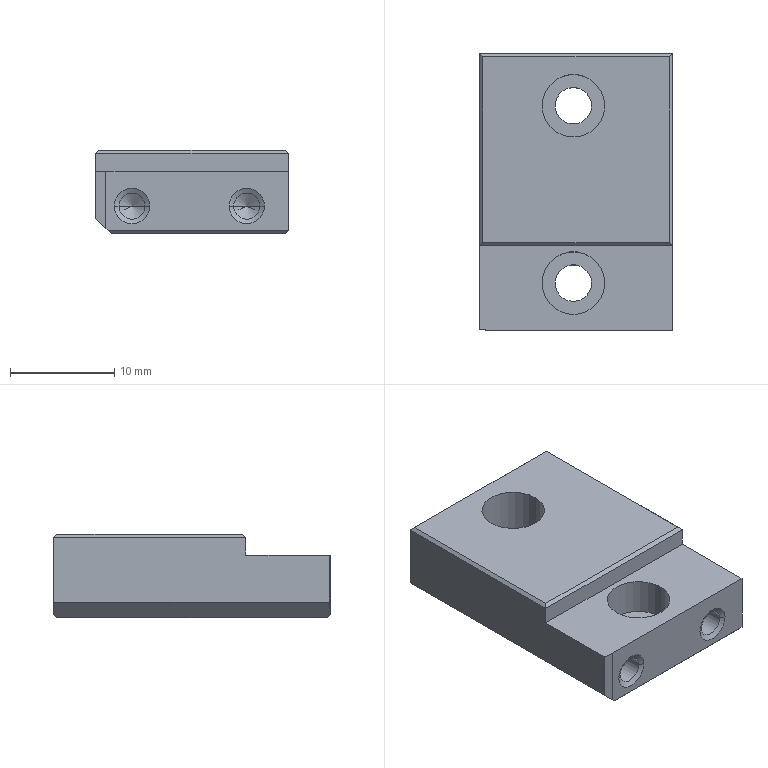Part | NX | 1 solid | 39 faces | box 18.5 x 26.53 x 8 mm | volume 3216 mm3 | plane 19 | cylinder 12 | cone 8 | commonest cylinder face diameters 2.5 x4 3.5 x4 6 x4
STEP:
#1=CARTESIAN_POINT('',(0.3,26.23,8.));
#2=VERTEX_POINT('',#1);
#3=CARTESIAN_POINT('',(0.3,8.4,8.));
#4=VERTEX_POINT('',#3);
#5=CARTESIAN_POINT('',(0.3,0.,8.));
#6=DIRECTION('',(0.,-1.,0.));
#7=VECTOR('',#6,1000.);
#8=LINE('',#5,#7);
#9=EDGE_CURVE('',#2,#4,#8,.T.);
#10=ORIENTED_EDGE('',*,*,#9,.T.);
#11=CARTESIAN_POINT('',(18.2,8.4,8.));
#12=VERTEX_POINT('',#11);
#13=CARTESIAN_POINT('',(0.,8.4,8.));
#14=DIRECTION('',(-1.,0.,0.));
#15=VECTOR('',#14,1000.);
#16=LINE('',#13,#15);
#17=EDGE_CURVE('',#12,#4,#16,.T.);
#18=ORIENTED_EDGE('',*,*,#17,.F.);
#19=CARTESIAN_POINT('',(18.2,26.23,8.));
#20=VERTEX_POINT('',#19);
#21=CARTESIAN_POINT('',(18.2,0.,8.));
#22=DIRECTION('',(0.,-1.,0.));
#23=VECTOR('',#22,1000.);
#24=LINE('',#21,#23);
#25=EDGE_CURVE('',#20,#12,#24,.T.);
#26=ORIENTED_EDGE('',*,*,#25,.F.);
#27=CARTESIAN_POINT('',(0.,26.23,8.));
#28=DIRECTION('',(1.,0.,0.));
#29=VECTOR('',#28,1000.);
#30=LINE('',#27,#29);
#31=EDGE_CURVE('',#2,#20,#30,.T.);
#32=ORIENTED_EDGE('',*,*,#31,.F.);
#33=EDGE_LOOP('',(#10,#18,#26,#32));
#34=FACE_BOUND('',#33,.T.);
#35=CARTESIAN_POINT('',(12.,21.53,8.));
#36=VERTEX_POINT('',#35);
#37=CARTESIAN_POINT('',(6.,21.53,8.));
#38=VERTEX_POINT('',#37);
#39=CARTESIAN_POINT('',(9.,21.53,8.));
#40=DIRECTION('',(0.,0.,1.));
#41=DIRECTION('',(1.,0.,0.));
#42=AXIS2_PLACEMENT_3D('',#39,#40,#41);
#43=CIRCLE('',#42,3.);
#44=EDGE_CURVE('',#36,#38,#43,.T.);
#45=ORIENTED_EDGE('',*,*,#44,.F.);
#46=CARTESIAN_POINT('',(9.,21.53,8.));
#47=DIRECTION('',(0.,0.,1.));
#48=DIRECTION('',(1.,0.,0.));
#49=AXIS2_PLACEMENT_3D('',#46,#47,#48);
#50=CIRCLE('',#49,3.);
#51=EDGE_CURVE('',#38,#36,#50,.T.);
#52=ORIENTED_EDGE('',*,*,#51,.F.);
#53=EDGE_LOOP('',(#45,#52));
#54=FACE_BOUND('',#53,.T.);
#55=CARTESIAN_POINT('',(0.,0.,8.));
#56=DIRECTION('',(0.,0.,1.));
#57=DIRECTION('',(1.,0.,0.));
#58=AXIS2_PLACEMENT_3D('',#55,#56,#57);
#59=PLANE('',#58);
#60=ADVANCED_FACE('',(#34,#54),#59,.T.);
#61=CARTESIAN_POINT('',(12.,4.53,2.5));
#62=VERTEX_POINT('',#61);
#63=CARTESIAN_POINT('',(6.,4.53,2.5));
#64=VERTEX_POINT('',#63);
#65=CARTESIAN_POINT('',(9.,4.53,2.5));
#66=DIRECTION('',(0.,0.,1.));
#67=DIRECTION('',(-1.,0.,0.));
#68=AXIS2_PLACEMENT_3D('',#65,#66,#67);
#69=CIRCLE('',#68,3.);
#70=EDGE_CURVE('',#62,#64,#69,.T.);
#71=ORIENTED_EDGE('',*,*,#70,.T.);
#72=CARTESIAN_POINT('',(9.,4.53,2.5));
#73=DIRECTION('',(0.,0.,1.));
#74=DIRECTION('',(-1.,0.,0.));
#75=AXIS2_PLACEMENT_3D('',#72,#73,#74);
#76=CIRCLE('',#75,3.);
#77=EDGE_CURVE('',#64,#62,#76,.T.);
#78=ORIENTED_EDGE('',*,*,#77,.T.);
#79=EDGE_LOOP('',(#71,#78));
#80=FACE_BOUND('',#79,.T.);
#81=CARTESIAN_POINT('',(7.25,4.53,2.5));
#82=VERTEX_POINT('',#81);
#83=CARTESIAN_POINT('',(10.75,4.53,2.5));
#84=VERTEX_POINT('',#83);
#85=CARTESIAN_POINT('',(9.,4.53,2.5));
#86=DIRECTION('',(0.,0.,1.));
#87=DIRECTION('',(-1.,0.,0.));
#88=AXIS2_PLACEMENT_3D('',#85,#86,#87);
#89=CIRCLE('',#88,1.75);
#90=EDGE_CURVE('',#82,#84,#89,.T.);
#91=ORIENTED_EDGE('',*,*,#90,.F.);
#92=CARTESIAN_POINT('',(9.,4.53,2.5));
#93=DIRECTION('',(0.,0.,1.));
#94=DIRECTION('',(-1.,0.,0.));
#95=AXIS2_PLACEMENT_3D('',#92,#93,#94);
#96=CIRCLE('',#95,1.75);
#97=EDGE_CURVE('',#84,#82,#96,.T.);
#98=ORIENTED_EDGE('',*,*,#97,.F.);
#99=EDGE_LOOP('',(#91,#98));
#100=FACE_BOUND('',#99,.T.);
#101=CARTESIAN_POINT('',(9.,4.53,2.5));
#102=DIRECTION('',(0.,0.,1.));
#103=DIRECTION('',(1.,0.,0.));
#104=AXIS2_PLACEMENT_3D('',#101,#102,#103);
#105=PLANE('',#104);
#106=ADVANCED_FACE('',(#80,#100),#105,.T.);
#107=CARTESIAN_POINT('',(18.5,0.,6.));
#108=VERTEX_POINT('',#107);
#109=CARTESIAN_POINT('',(1.,0.,6.));
#110=VERTEX_POINT('',#109);
#111=CARTESIAN_POINT('',(0.,0.,6.));
#112=DIRECTION('',(-1.,0.,0.));
#113=VECTOR('',#112,1000.);
#114=LINE('',#111,#113);
#115=EDGE_CURVE('',#108,#110,#114,.T.);
#116=ORIENTED_EDGE('',*,*,#115,.T.);
#117=CARTESIAN_POINT('',(1.,0.,0.5));
#118=VERTEX_POINT('',#117);
#119=CARTESIAN_POINT('',(1.,0.,0.));
#120=DIRECTION('',(0.,0.,1.));
#121=VECTOR('',#120,1000.);
#122=LINE('',#119,#121);
#123=EDGE_CURVE('',#118,#110,#122,.T.);
#124=ORIENTED_EDGE('',*,*,#123,.F.);
#125=CARTESIAN_POINT('',(1.2,0.,0.3));
#126=VERTEX_POINT('',#125);
#127=CARTESIAN_POINT('',(1.5,0.,0.));
#128=DIRECTION('',(-0.7071,0.,0.7071));
#129=VECTOR('',#128,1000.);
#130=LINE('',#127,#129);
#131=EDGE_CURVE('',#126,#118,#130,.T.);
#132=ORIENTED_EDGE('',*,*,#131,.F.);
#133=CARTESIAN_POINT('',(18.5,0.,0.3));
#134=VERTEX_POINT('',#133);
#135=CARTESIAN_POINT('',(0.,0.,0.3));
#136=DIRECTION('',(1.,0.,0.));
#137=VECTOR('',#136,1000.);
#138=LINE('',#135,#137);
#139=EDGE_CURVE('',#126,#134,#138,.T.);
#140=ORIENTED_EDGE('',*,*,#139,.T.);
#141=CARTESIAN_POINT('',(18.5,0.,0.));
#142=DIRECTION('',(0.,0.,-1.));
#143=VECTOR('',#142,1000.);
#144=LINE('',#141,#143);
#145=EDGE_CURVE('',#108,#134,#144,.T.);
#146=ORIENTED_EDGE('',*,*,#145,.F.);
#147=EDGE_LOOP('',(#116,#124,#132,#140,#146));
#148=FACE_BOUND('',#147,.T.);
#149=CARTESIAN_POINT('',(12.8,0.,2.65));
#150=VERTEX_POINT('',#149);
#151=CARTESIAN_POINT('',(16.2,0.,2.65));
#152=VERTEX_POINT('',#151);
#153=CARTESIAN_POINT('',(14.5,0.,2.65));
#154=DIRECTION('',(0.,-1.,0.));
#155=DIRECTION('',(-1.,0.,0.));
#156=AXIS2_PLACEMENT_3D('',#153,#154,#155);
#157=CIRCLE('',#156,1.7);
#158=EDGE_CURVE('',#150,#152,#157,.T.);
#159=ORIENTED_EDGE('',*,*,#158,.F.);
#160=CARTESIAN_POINT('',(14.5,0.,2.65));
#161=DIRECTION('',(0.,-1.,0.));
#162=DIRECTION('',(-1.,0.,0.));
#163=AXIS2_PLACEMENT_3D('',#160,#161,#162);
#164=CIRCLE('',#163,1.7);
#165=EDGE_CURVE('',#152,#150,#164,.T.);
#166=ORIENTED_EDGE('',*,*,#165,.F.);
#167=EDGE_LOOP('',(#159,#166));
#168=FACE_BOUND('',#167,.T.);
#169=CARTESIAN_POINT('',(1.8,0.,2.65));
#170=VERTEX_POINT('',#169);
#171=CARTESIAN_POINT('',(5.2,0.,2.65));
#172=VERTEX_POINT('',#171);
#173=CARTESIAN_POINT('',(3.5,0.,2.65));
#174=DIRECTION('',(0.,-1.,0.));
#175=DIRECTION('',(-1.,0.,0.));
#176=AXIS2_PLACEMENT_3D('',#173,#174,#175);
#177=CIRCLE('',#176,1.7);
#178=EDGE_CURVE('',#170,#172,#177,.T.);
#179=ORIENTED_EDGE('',*,*,#178,.F.);
#180=CARTESIAN_POINT('',(3.5,0.,2.65));
#181=DIRECTION('',(0.,-1.,0.));
#182=DIRECTION('',(-1.,0.,0.));
#183=AXIS2_PLACEMENT_3D('',#180,#181,#182);
#184=CIRCLE('',#183,1.7);
#185=EDGE_CURVE('',#172,#170,#184,.T.);
#186=ORIENTED_EDGE('',*,*,#185,.F.);
#187=EDGE_LOOP('',(#179,#186));
#188=FACE_BOUND('',#187,.T.);
#189=CARTESIAN_POINT('',(0.,0.,0.));
#190=DIRECTION('',(0.,-1.,0.));
#191=DIRECTION('',(0.,0.,-1.));
#192=AXIS2_PLACEMENT_3D('',#189,#190,#191);
#193=PLANE('',#192);
#194=ADVANCED_FACE('',(#148,#168,#188),#193,.T.);
#195=ORIENTED_EDGE('',*,*,#123,.T.);
#196=CARTESIAN_POINT('',(0.,0.08749,6.));
#197=VERTEX_POINT('',#196);
#198=CARTESIAN_POINT('',(0.,0.08749,6.));
#199=DIRECTION('',(0.9962,-0.08716,0.));
#200=VECTOR('',#199,1000.);
#201=LINE('',#198,#200);
#202=EDGE_CURVE('',#197,#110,#201,.T.);
#203=ORIENTED_EDGE('',*,*,#202,.F.);
#204=CARTESIAN_POINT('',(0.,0.08749,1.5));
#205=VERTEX_POINT('',#204);
#206=CARTESIAN_POINT('',(0.,0.08749,0.));
#207=DIRECTION('',(0.,0.,-1.));
#208=VECTOR('',#207,1000.);
#209=LINE('',#206,#208);
#210=EDGE_CURVE('',#197,#205,#209,.T.);
#211=ORIENTED_EDGE('',*,*,#210,.T.);
#212=CARTESIAN_POINT('',(0.,0.08749,1.5));
#213=DIRECTION('',(-0.7058,0.06175,0.7058));
#214=VECTOR('',#213,1000.);
#215=LINE('',#212,#214);
#216=EDGE_CURVE('',#118,#205,#215,.T.);
#217=ORIENTED_EDGE('',*,*,#216,.F.);
#218=EDGE_LOOP('',(#195,#203,#211,#217));
#219=FACE_BOUND('',#218,.T.);
#220=CARTESIAN_POINT('',(1.,0.,0.5));
#221=DIRECTION('',(-0.08716,-0.9962,0.));
#222=DIRECTION('',(-0.9962,0.08716,0.));
#223=AXIS2_PLACEMENT_3D('',#220,#221,#222);
#224=PLANE('',#223);
#225=ADVANCED_FACE('',(#219),#224,.T.);
#226=CARTESIAN_POINT('',(1.5,0.3,0.));
#227=VERTEX_POINT('',#226);
#228=CARTESIAN_POINT('',(1.5,26.23,0.));
#229=VERTEX_POINT('',#228);
#230=CARTESIAN_POINT('',(1.5,0.,0.));
#231=DIRECTION('',(0.,1.,0.));
#232=VECTOR('',#231,1000.);
#233=LINE('',#230,#232);
#234=EDGE_CURVE('',#227,#229,#233,.T.);
#235=ORIENTED_EDGE('',*,*,#234,.F.);
#236=CARTESIAN_POINT('',(1.5,0.3,0.));
#237=DIRECTION('',(-0.5774,-0.5774,0.5774));
#238=VECTOR('',#237,1000.);
#239=LINE('',#236,#238);
#240=EDGE_CURVE('',#227,#126,#239,.T.);
#241=ORIENTED_EDGE('',*,*,#240,.T.);
#242=ORIENTED_EDGE('',*,*,#131,.T.);
#243=ORIENTED_EDGE('',*,*,#216,.T.);
#244=CARTESIAN_POINT('',(0.,26.53,1.5));
#245=VERTEX_POINT('',#244);
#246=CARTESIAN_POINT('',(0.,0.,1.5));
#247=DIRECTION('',(0.,1.,0.));
#248=VECTOR('',#247,1000.);
#249=LINE('',#246,#248);
#250=EDGE_CURVE('',#205,#245,#249,.T.);
#251=ORIENTED_EDGE('',*,*,#250,.T.);
#252=CARTESIAN_POINT('',(1.2,26.53,0.3));
#253=VERTEX_POINT('',#252);
#254=CARTESIAN_POINT('',(0.,26.53,1.5));
#255=DIRECTION('',(0.7071,0.,-0.7071));
#256=VECTOR('',#255,1000.);
#257=LINE('',#254,#256);
#258=EDGE_CURVE('',#245,#253,#257,.T.);
#259=ORIENTED_EDGE('',*,*,#258,.T.);
#260=CARTESIAN_POINT('',(27.73,0.,-26.23));
#261=DIRECTION('',(-0.5774,0.5774,0.5774));
#262=VECTOR('',#261,1000.);
#263=LINE('',#260,#262);
#264=EDGE_CURVE('',#229,#253,#263,.T.);
#265=ORIENTED_EDGE('',*,*,#264,.F.);
#266=EDGE_LOOP('',(#235,#241,#242,#243,#251,#259,#265));
#267=FACE_BOUND('',#266,.T.);
#268=CARTESIAN_POINT('',(1.5,26.53,0.));
#269=DIRECTION('',(-0.7071,0.,-0.7071));
#270=DIRECTION('',(-0.7071,0.,0.7071));
#271=AXIS2_PLACEMENT_3D('',#268,#269,#270);
#272=PLANE('',#271);
#273=ADVANCED_FACE('',(#267),#272,.T.);
#274=CARTESIAN_POINT('',(18.5,26.53,7.7));
#275=VERTEX_POINT('',#274);
#276=CARTESIAN_POINT('',(0.,26.53,7.7));
#277=VERTEX_POINT('',#276);
#278=CARTESIAN_POINT('',(0.,26.53,7.7));
#279=DIRECTION('',(-1.,0.,0.));
#280=VECTOR('',#279,1000.);
#281=LINE('',#278,#280);
#282=EDGE_CURVE('',#275,#277,#281,.T.);
#283=ORIENTED_EDGE('',*,*,#282,.F.);
#284=CARTESIAN_POINT('',(18.5,26.53,0.3));
#285=VERTEX_POINT('',#284);
#286=CARTESIAN_POINT('',(18.5,26.53,0.));
#287=DIRECTION('',(0.,0.,-1.));
#288=VECTOR('',#287,1000.);
#289=LINE('',#286,#288);
#290=EDGE_CURVE('',#275,#285,#289,.T.);
#291=ORIENTED_EDGE('',*,*,#290,.T.);
#292=CARTESIAN_POINT('',(0.,26.53,0.3));
#293=DIRECTION('',(1.,0.,0.));
#294=VECTOR('',#293,1000.);
#295=LINE('',#292,#294);
#296=EDGE_CURVE('',#253,#285,#295,.T.);
#297=ORIENTED_EDGE('',*,*,#296,.F.);
#298=ORIENTED_EDGE('',*,*,#258,.F.);
#299=CARTESIAN_POINT('',(0.,26.53,0.));
#300=DIRECTION('',(0.,0.,1.));
#301=VECTOR('',#300,1000.);
#302=LINE('',#299,#301);
#303=EDGE_CURVE('',#245,#277,#302,.T.);
#304=ORIENTED_EDGE('',*,*,#303,.T.);
#305=EDGE_LOOP('',(#283,#291,#297,#298,#304));
#306=FACE_BOUND('',#305,.T.);
#307=CARTESIAN_POINT('',(18.5,26.53,0.));
#308=DIRECTION('',(0.,1.,0.));
#309=DIRECTION('',(1.,0.,0.));
#310=AXIS2_PLACEMENT_3D('',#307,#308,#309);
#311=PLANE('',#310);
#312=ADVANCED_FACE('',(#306),#311,.T.);
#313=CARTESIAN_POINT('',(18.5,8.1,7.7));
#314=VERTEX_POINT('',#313);
#315=CARTESIAN_POINT('',(18.5,0.,7.7));
#316=DIRECTION('',(0.,1.,0.));
#317=VECTOR('',#316,1000.);
#318=LINE('',#315,#317);
#319=EDGE_CURVE('',#314,#275,#318,.T.);
#320=ORIENTED_EDGE('',*,*,#319,.F.);
#321=CARTESIAN_POINT('',(18.5,8.1,6.));
#322=VERTEX_POINT('',#321);
#323=CARTESIAN_POINT('',(18.5,8.1,0.));
#324=DIRECTION('',(0.,0.,-1.));
#325=VECTOR('',#324,1000.);
#326=LINE('',#323,#325);
#327=EDGE_CURVE('',#314,#322,#326,.T.);
#328=ORIENTED_EDGE('',*,*,#327,.T.);
#329=CARTESIAN_POINT('',(18.5,0.,6.));
#330=DIRECTION('',(0.,1.,0.));
#331=VECTOR('',#330,1000.);
#332=LINE('',#329,#331);
#333=EDGE_CURVE('',#108,#322,#332,.T.);
#334=ORIENTED_EDGE('',*,*,#333,.F.);
#335=ORIENTED_EDGE('',*,*,#145,.T.);
#336=CARTESIAN_POINT('',(18.5,0.,0.3));
#337=DIRECTION('',(0.,-1.,0.));
#338=VECTOR('',#337,1000.);
#339=LINE('',#336,#338);
#340=EDGE_CURVE('',#285,#134,#339,.T.);
#341=ORIENTED_EDGE('',*,*,#340,.F.);
#342=ORIENTED_EDGE('',*,*,#290,.F.);
#343=EDGE_LOOP('',(#320,#328,#334,#335,#341,#342));
#344=FACE_BOUND('',#343,.T.);
#345=CARTESIAN_POINT('',(18.5,0.,0.));
#346=DIRECTION('',(1.,0.,0.));
#347=DIRECTION('',(0.,1.,0.));
#348=AXIS2_PLACEMENT_3D('',#345,#346,#347);
#349=PLANE('',#348);
#350=ADVANCED_FACE('',(#344),#349,.T.);
#351=CARTESIAN_POINT('',(0.,8.1,7.7));
#352=VERTEX_POINT('',#351);
#353=CARTESIAN_POINT('',(0.,8.1,7.7));
#354=DIRECTION('',(-1.,0.,0.));
#355=VECTOR('',#354,1000.);
#356=LINE('',#353,#355);
#357=EDGE_CURVE('',#314,#352,#356,.T.);
#358=ORIENTED_EDGE('',*,*,#357,.T.);
#359=CARTESIAN_POINT('',(0.,8.1,6.));
#360=VERTEX_POINT('',#359);
#361=CARTESIAN_POINT('',(0.,8.1,0.));
#362=DIRECTION('',(0.,0.,1.));
#363=VECTOR('',#362,1000.);
#364=LINE('',#361,#363);
#365=EDGE_CURVE('',#360,#352,#364,.T.);
#366=ORIENTED_EDGE('',*,*,#365,.F.);
#367=CARTESIAN_POINT('',(0.,8.1,6.));
#368=DIRECTION('',(-1.,0.,0.));
#369=VECTOR('',#368,1000.);
#370=LINE('',#367,#369);
#371=EDGE_CURVE('',#322,#360,#370,.T.);
#372=ORIENTED_EDGE('',*,*,#371,.F.);
#373=ORIENTED_EDGE('',*,*,#327,.F.);
#374=EDGE_LOOP('',(#358,#366,#372,#373));
#375=FACE_BOUND('',#374,.T.);
#376=CARTESIAN_POINT('',(18.5,8.1,5.85));
#377=DIRECTION('',(0.,1.,0.));
#378=DIRECTION('',(1.,0.,0.));
#379=AXIS2_PLACEMENT_3D('',#376,#377,#378);
#380=PLANE('',#379);
#381=ADVANCED_FACE('',(#375),#380,.F.);
#382=CARTESIAN_POINT('',(18.2,26.23,0.));
#383=VERTEX_POINT('',#382);
#384=CARTESIAN_POINT('',(18.2,0.3,0.));
#385=VERTEX_POINT('',#384);
#386=CARTESIAN_POINT('',(18.2,0.,0.));
#387=DIRECTION('',(0.,-1.,0.));
#388=VECTOR('',#387,1000.);
#389=LINE('',#386,#388);
#390=EDGE_CURVE('',#383,#385,#389,.T.);
#391=ORIENTED_EDGE('',*,*,#390,.T.);
#392=CARTESIAN_POINT('',(0.,0.3,0.));
#393=DIRECTION('',(1.,0.,0.));
#394=VECTOR('',#393,1000.);
#395=LINE('',#392,#394);
#396=EDGE_CURVE('',#227,#385,#395,.T.);
#397=ORIENTED_EDGE('',*,*,#396,.F.);
#398=ORIENTED_EDGE('',*,*,#234,.T.);
#399=CARTESIAN_POINT('',(0.,26.23,0.));
#400=DIRECTION('',(1.,0.,0.));
#401=VECTOR('',#400,1000.);
#402=LINE('',#399,#401);
#403=EDGE_CURVE('',#229,#383,#402,.T.);
#404=ORIENTED_EDGE('',*,*,#403,.T.);
#405=EDGE_LOOP('',(#391,#397,#398,#404));
#406=FACE_BOUND('',#405,.T.);
#407=CARTESIAN_POINT('',(10.75,21.53,0.));
#408=VERTEX_POINT('',#407);
#409=CARTESIAN_POINT('',(7.25,21.53,0.));
#410=VERTEX_POINT('',#409);
#411=CARTESIAN_POINT('',(9.,21.53,0.));
#412=DIRECTION('',(0.,0.,-1.));
#413=DIRECTION('',(-1.,0.,0.));
#414=AXIS2_PLACEMENT_3D('',#411,#412,#413);
#415=CIRCLE('',#414,1.75);
#416=EDGE_CURVE('',#408,#410,#415,.T.);
#417=ORIENTED_EDGE('',*,*,#416,.F.);
#418=CARTESIAN_POINT('',(9.,21.53,0.));
#419=DIRECTION('',(0.,0.,-1.));
#420=DIRECTION('',(-1.,0.,0.));
#421=AXIS2_PLACEMENT_3D('',#418,#419,#420);
#422=CIRCLE('',#421,1.75);
#423=EDGE_CURVE('',#410,#408,#422,.T.);
#424=ORIENTED_EDGE('',*,*,#423,.F.);
#425=EDGE_LOOP('',(#417,#424));
#426=FACE_BOUND('',#425,.T.);
#427=CARTESIAN_POINT('',(7.25,4.53,0.));
#428=VERTEX_POINT('',#427);
#429=CARTESIAN_POINT('',(10.75,4.53,0.));
#430=VERTEX_POINT('',#429);
#431=CARTESIAN_POINT('',(9.,4.53,0.));
#432=DIRECTION('',(0.,0.,-1.));
#433=DIRECTION('',(-1.,0.,0.));
#434=AXIS2_PLACEMENT_3D('',#431,#432,#433);
#435=CIRCLE('',#434,1.75);
#436=EDGE_CURVE('',#428,#430,#435,.T.);
#437=ORIENTED_EDGE('',*,*,#436,.F.);
#438=CARTESIAN_POINT('',(9.,4.53,0.));
#439=DIRECTION('',(0.,0.,-1.));
#440=DIRECTION('',(-1.,0.,0.));
#441=AXIS2_PLACEMENT_3D('',#438,#439,#440);
#442=CIRCLE('',#441,1.75);
#443=EDGE_CURVE('',#430,#428,#442,.T.);
#444=ORIENTED_EDGE('',*,*,#443,.F.);
#445=EDGE_LOOP('',(#437,#444));
#446=FACE_BOUND('',#445,.T.);
#447=CARTESIAN_POINT('',(0.,0.,0.));
#448=DIRECTION('',(0.,0.,1.));
#449=DIRECTION('',(1.,0.,0.));
#450=AXIS2_PLACEMENT_3D('',#447,#448,#449);
#451=PLANE('',#450);
#452=ADVANCED_FACE('',(#406,#426,#446),#451,.F.);
#453=CARTESIAN_POINT('',(0.,0.,6.));
#454=DIRECTION('',(0.,1.,0.));
#455=VECTOR('',#454,1000.);
#456=LINE('',#453,#455);
#457=EDGE_CURVE('',#197,#360,#456,.T.);
#458=ORIENTED_EDGE('',*,*,#457,.T.);
#459=ORIENTED_EDGE('',*,*,#365,.T.);
#460=CARTESIAN_POINT('',(0.,0.,7.7));
#461=DIRECTION('',(0.,1.,0.));
#462=VECTOR('',#461,1000.);
#463=LINE('',#460,#462);
#464=EDGE_CURVE('',#352,#277,#463,.T.);
#465=ORIENTED_EDGE('',*,*,#464,.T.);
#466=ORIENTED_EDGE('',*,*,#303,.F.);
#467=ORIENTED_EDGE('',*,*,#250,.F.);
#468=ORIENTED_EDGE('',*,*,#210,.F.);
#469=EDGE_LOOP('',(#458,#459,#465,#466,#467,#468));
#470=FACE_BOUND('',#469,.T.);
#471=CARTESIAN_POINT('',(0.,26.53,0.));
#472=DIRECTION('',(-1.,0.,0.));
#473=DIRECTION('',(0.,0.,1.));
#474=AXIS2_PLACEMENT_3D('',#471,#472,#473);
#475=PLANE('',#474);
#476=ADVANCED_FACE('',(#470),#475,.T.);
#477=ORIENTED_EDGE('',*,*,#44,.T.);
#478=CARTESIAN_POINT('',(6.,21.53,2.5));
#479=VERTEX_POINT('',#478);
#480=CARTESIAN_POINT('',(6.,21.53,-1.24));
#481=DIRECTION('',(0.,0.,1.));
#482=VECTOR('',#481,1000.);
#483=LINE('',#480,#482);
#484=EDGE_CURVE('',#38,#479,#483,.F.);
#485=ORIENTED_EDGE('',*,*,#484,.T.);
#486=CARTESIAN_POINT('',(12.,21.53,2.5));
#487=VERTEX_POINT('',#486);
#488=CARTESIAN_POINT('',(9.,21.53,2.5));
#489=DIRECTION('',(0.,0.,-1.));
#490=DIRECTION('',(-1.,0.,0.));
#491=AXIS2_PLACEMENT_3D('',#488,#489,#490);
#492=CIRCLE('',#491,3.);
#493=EDGE_CURVE('',#479,#487,#492,.T.);
#494=ORIENTED_EDGE('',*,*,#493,.T.);
#495=CARTESIAN_POINT('',(12.,21.53,-1.24));
#496=DIRECTION('',(0.,0.,1.));
#497=VECTOR('',#496,1000.);
#498=LINE('',#495,#497);
#499=EDGE_CURVE('',#36,#487,#498,.F.);
#500=ORIENTED_EDGE('',*,*,#499,.F.);
#501=EDGE_LOOP('',(#477,#485,#494,#500));
#502=FACE_BOUND('',#501,.T.);
#503=CARTESIAN_POINT('',(9.,21.53,-1.24));
#504=DIRECTION('',(0.,0.,1.));
#505=DIRECTION('',(-1.,0.,0.));
#506=AXIS2_PLACEMENT_3D('',#503,#504,#505);
#507=CYLINDRICAL_SURFACE('',#506,3.);
#508=ADVANCED_FACE('',(#502),#507,.F.);
#509=ORIENTED_EDGE('',*,*,#115,.F.);
#510=ORIENTED_EDGE('',*,*,#333,.T.);
#511=ORIENTED_EDGE('',*,*,#371,.T.);
#512=ORIENTED_EDGE('',*,*,#457,.F.);
#513=ORIENTED_EDGE('',*,*,#202,.T.);
#514=EDGE_LOOP('',(#509,#510,#511,#512,#513));
#515=FACE_BOUND('',#514,.T.);
#516=CARTESIAN_POINT('',(6.,4.53,6.));
#517=VERTEX_POINT('',#516);
#518=CARTESIAN_POINT('',(12.,4.53,6.));
#519=VERTEX_POINT('',#518);
#520=CARTESIAN_POINT('',(9.,4.53,6.));
#521=DIRECTION('',(0.,0.,1.));
#522=DIRECTION('',(-1.,0.,0.));
#523=AXIS2_PLACEMENT_3D('',#520,#521,#522);
#524=CIRCLE('',#523,3.);
#525=EDGE_CURVE('',#517,#519,#524,.T.);
#526=ORIENTED_EDGE('',*,*,#525,.F.);
#527=CARTESIAN_POINT('',(9.,4.53,6.));
#528=DIRECTION('',(0.,0.,1.));
#529=DIRECTION('',(-1.,0.,0.));
#530=AXIS2_PLACEMENT_3D('',#527,#528,#529);
#531=CIRCLE('',#530,3.);
#532=EDGE_CURVE('',#519,#517,#531,.T.);
#533=ORIENTED_EDGE('',*,*,#532,.F.);
#534=EDGE_LOOP('',(#526,#533));
#535=FACE_BOUND('',#534,.T.);
#536=CARTESIAN_POINT('',(18.5,0.,6.));
#537=DIRECTION('',(0.,0.,-1.));
#538=DIRECTION('',(0.,-1.,0.));
#539=AXIS2_PLACEMENT_3D('',#536,#537,#538);
#540=PLANE('',#539);
#541=ADVANCED_FACE('',(#515,#535),#540,.F.);
#542=CARTESIAN_POINT('',(9.,21.53,2.5));
#543=DIRECTION('',(0.,0.,-1.));
#544=DIRECTION('',(-1.,0.,0.));
#545=AXIS2_PLACEMENT_3D('',#542,#543,#544);
#546=CIRCLE('',#545,3.);
#547=EDGE_CURVE('',#487,#479,#546,.T.);
#548=ORIENTED_EDGE('',*,*,#547,.F.);
#549=ORIENTED_EDGE('',*,*,#493,.F.);
#550=EDGE_LOOP('',(#548,#549));
#551=FACE_BOUND('',#550,.T.);
#552=CARTESIAN_POINT('',(7.25,21.53,2.5));
#553=VERTEX_POINT('',#552);
#554=CARTESIAN_POINT('',(10.75,21.53,2.5));
#555=VERTEX_POINT('',#554);
#556=CARTESIAN_POINT('',(9.,21.53,2.5));
#557=DIRECTION('',(0.,0.,1.));
#558=DIRECTION('',(-1.,0.,0.));
#559=AXIS2_PLACEMENT_3D('',#556,#557,#558);
#560=CIRCLE('',#559,1.75);
#561=EDGE_CURVE('',#553,#555,#560,.T.);
#562=ORIENTED_EDGE('',*,*,#561,.F.);
#563=CARTESIAN_POINT('',(9.,21.53,2.5));
#564=DIRECTION('',(0.,0.,1.));
#565=DIRECTION('',(-1.,0.,0.));
#566=AXIS2_PLACEMENT_3D('',#563,#564,#565);
#567=CIRCLE('',#566,1.75);
#568=EDGE_CURVE('',#555,#553,#567,.T.);
#569=ORIENTED_EDGE('',*,*,#568,.F.);
#570=EDGE_LOOP('',(#562,#569));
#571=FACE_BOUND('',#570,.T.);
#572=CARTESIAN_POINT('',(9.,21.53,2.5));
#573=DIRECTION('',(0.,0.,1.));
#574=DIRECTION('',(1.,0.,0.));
#575=AXIS2_PLACEMENT_3D('',#572,#573,#574);
#576=PLANE('',#575);
#577=ADVANCED_FACE('',(#551,#571),#576,.T.);
#578=ORIENTED_EDGE('',*,*,#561,.T.);
#579=CARTESIAN_POINT('',(10.75,21.53,-1.24));
#580=DIRECTION('',(0.,0.,1.));
#581=VECTOR('',#580,1000.);
#582=LINE('',#579,#581);
#583=EDGE_CURVE('',#555,#408,#582,.F.);
#584=ORIENTED_EDGE('',*,*,#583,.T.);
#585=ORIENTED_EDGE('',*,*,#416,.T.);
#586=CARTESIAN_POINT('',(7.25,21.53,-1.24));
#587=DIRECTION('',(0.,0.,1.));
#588=VECTOR('',#587,1000.);
#589=LINE('',#586,#588);
#590=EDGE_CURVE('',#553,#410,#589,.F.);
#591=ORIENTED_EDGE('',*,*,#590,.F.);
#592=EDGE_LOOP('',(#578,#584,#585,#591));
#593=FACE_BOUND('',#592,.T.);
#594=CARTESIAN_POINT('',(9.,21.53,-1.24));
#595=DIRECTION('',(0.,0.,1.));
#596=DIRECTION('',(-1.,0.,0.));
#597=AXIS2_PLACEMENT_3D('',#594,#595,#596);
#598=CYLINDRICAL_SURFACE('',#597,1.75);
#599=ADVANCED_FACE('',(#593),#598,.F.);
#600=ORIENTED_EDGE('',*,*,#90,.T.);
#601=CARTESIAN_POINT('',(10.75,4.53,-1.24));
#602=DIRECTION('',(0.,0.,1.));
#603=VECTOR('',#602,1000.);
#604=LINE('',#601,#603);
#605=EDGE_CURVE('',#430,#84,#604,.T.);
#606=ORIENTED_EDGE('',*,*,#605,.F.);
#607=ORIENTED_EDGE('',*,*,#443,.T.);
#608=CARTESIAN_POINT('',(7.25,4.53,-1.24));
#609=DIRECTION('',(0.,0.,1.));
#610=VECTOR('',#609,1000.);
#611=LINE('',#608,#610);
#612=EDGE_CURVE('',#428,#82,#611,.T.);
#613=ORIENTED_EDGE('',*,*,#612,.T.);
#614=EDGE_LOOP('',(#600,#606,#607,#613));
#615=FACE_BOUND('',#614,.T.);
#616=CARTESIAN_POINT('',(9.,4.53,-1.24));
#617=DIRECTION('',(0.,0.,1.));
#618=DIRECTION('',(-1.,0.,0.));
#619=AXIS2_PLACEMENT_3D('',#616,#617,#618);
#620=CYLINDRICAL_SURFACE('',#619,1.75);
#621=ADVANCED_FACE('',(#615),#620,.F.);
#622=ORIENTED_EDGE('',*,*,#70,.F.);
#623=CARTESIAN_POINT('',(12.,4.53,-1.24));
#624=DIRECTION('',(0.,0.,1.));
#625=VECTOR('',#624,1000.);
#626=LINE('',#623,#625);
#627=EDGE_CURVE('',#62,#519,#626,.T.);
#628=ORIENTED_EDGE('',*,*,#627,.T.);
#629=ORIENTED_EDGE('',*,*,#532,.T.);
#630=CARTESIAN_POINT('',(6.,4.53,-1.24));
#631=DIRECTION('',(0.,0.,1.));
#632=VECTOR('',#631,1000.);
#633=LINE('',#630,#632);
#634=EDGE_CURVE('',#64,#517,#633,.T.);
#635=ORIENTED_EDGE('',*,*,#634,.F.);
#636=EDGE_LOOP('',(#622,#628,#629,#635));
#637=FACE_BOUND('',#636,.T.);
#638=CARTESIAN_POINT('',(9.,4.53,-1.24));
#639=DIRECTION('',(0.,0.,1.));
#640=DIRECTION('',(-1.,0.,0.));
#641=AXIS2_PLACEMENT_3D('',#638,#639,#640);
#642=CYLINDRICAL_SURFACE('',#641,3.);
#643=ADVANCED_FACE('',(#637),#642,.F.);
#644=CARTESIAN_POINT('',(15.75,0.2598,2.65));
#645=VERTEX_POINT('',#644);
#646=CARTESIAN_POINT('',(13.25,0.2598,2.65));
#647=VERTEX_POINT('',#646);
#648=CARTESIAN_POINT('',(14.5,0.2598,2.65));
#649=DIRECTION('',(0.,-1.,0.));
#650=DIRECTION('',(-1.,0.,0.));
#651=AXIS2_PLACEMENT_3D('',#648,#649,#650);
#652=CIRCLE('',#651,1.25);
#653=EDGE_CURVE('',#645,#647,#652,.T.);
#654=ORIENTED_EDGE('',*,*,#653,.T.);
#655=CARTESIAN_POINT('',(13.25,7.,2.65));
#656=VERTEX_POINT('',#655);
#657=CARTESIAN_POINT('',(13.25,0.,2.65));
#658=DIRECTION('',(0.,-1.,0.));
#659=VECTOR('',#658,1000.);
#660=LINE('',#657,#659);
#661=EDGE_CURVE('',#647,#656,#660,.F.);
#662=ORIENTED_EDGE('',*,*,#661,.T.);
#663=CARTESIAN_POINT('',(15.75,7.,2.65));
#664=VERTEX_POINT('',#663);
#665=CARTESIAN_POINT('',(14.5,7.,2.65));
#666=DIRECTION('',(0.,-1.,0.));
#667=DIRECTION('',(-1.,0.,0.));
#668=AXIS2_PLACEMENT_3D('',#665,#666,#667);
#669=CIRCLE('',#668,1.25);
#670=EDGE_CURVE('',#664,#656,#669,.T.);
#671=ORIENTED_EDGE('',*,*,#670,.F.);
#672=CARTESIAN_POINT('',(15.75,0.,2.65));
#673=DIRECTION('',(0.,-1.,0.));
#674=VECTOR('',#673,1000.);
#675=LINE('',#672,#674);
#676=EDGE_CURVE('',#645,#664,#675,.F.);
#677=ORIENTED_EDGE('',*,*,#676,.F.);
#678=EDGE_LOOP('',(#654,#662,#671,#677));
#679=FACE_BOUND('',#678,.T.);
#680=CARTESIAN_POINT('',(14.5,0.,2.65));
#681=DIRECTION('',(0.,-1.,0.));
#682=DIRECTION('',(-1.,0.,0.));
#683=AXIS2_PLACEMENT_3D('',#680,#681,#682);
#684=CYLINDRICAL_SURFACE('',#683,1.25);
#685=ADVANCED_FACE('',(#679),#684,.F.);
#686=ORIENTED_EDGE('',*,*,#319,.T.);
#687=CARTESIAN_POINT('',(-8.03,0.,34.23));
#688=DIRECTION('',(0.5774,0.5774,-0.5774));
#689=VECTOR('',#688,1000.);
#690=LINE('',#687,#689);
#691=EDGE_CURVE('',#20,#275,#690,.T.);
#692=ORIENTED_EDGE('',*,*,#691,.F.);
#693=ORIENTED_EDGE('',*,*,#25,.T.);
#694=CARTESIAN_POINT('',(26.6,0.,-0.4));
#695=DIRECTION('',(-0.5774,0.5774,0.5774));
#696=VECTOR('',#695,1000.);
#697=LINE('',#694,#696);
#698=EDGE_CURVE('',#314,#12,#697,.T.);
#699=ORIENTED_EDGE('',*,*,#698,.F.);
#700=EDGE_LOOP('',(#686,#692,#693,#699));
#701=FACE_BOUND('',#700,.T.);
#702=CARTESIAN_POINT('',(18.35,17.315,7.85));
#703=DIRECTION('',(0.7071,0.,0.7071));
#704=DIRECTION('',(0.,-1.,0.));
#705=AXIS2_PLACEMENT_3D('',#702,#703,#704);
#706=PLANE('',#705);
#707=ADVANCED_FACE('',(#701),#706,.T.);
#708=ORIENTED_EDGE('',*,*,#670,.T.);
#709=CARTESIAN_POINT('',(14.5,7.751,2.65));
#710=VERTEX_POINT('',#709);
#711=CARTESIAN_POINT('',(13.25,7.,2.65));
#712=DIRECTION('',(-0.8572,-0.515,0.));
#713=VECTOR('',#712,1000.);
#714=LINE('',#711,#713);
#715=EDGE_CURVE('',#710,#656,#714,.T.);
#716=ORIENTED_EDGE('',*,*,#715,.F.);
#717=CARTESIAN_POINT('',(15.75,7.,2.65));
#718=DIRECTION('',(0.8572,-0.515,0.));
#719=VECTOR('',#718,1000.);
#720=LINE('',#717,#719);
#721=EDGE_CURVE('',#710,#664,#720,.T.);
#722=ORIENTED_EDGE('',*,*,#721,.T.);
#723=EDGE_LOOP('',(#708,#716,#722));
#724=FACE_BOUND('',#723,.T.);
#725=CARTESIAN_POINT('',(14.5,7.,2.65));
#726=DIRECTION('',(0.,-1.,0.));
#727=DIRECTION('',(-1.,0.,0.));
#728=AXIS2_PLACEMENT_3D('',#725,#726,#727);
#729=CONICAL_SURFACE('',#728,1.25,1.03);
#730=ADVANCED_FACE('',(#724),#729,.F.);
#731=ORIENTED_EDGE('',*,*,#653,.F.);
#732=CARTESIAN_POINT('',(15.75,0.2598,2.65));
#733=DIRECTION('',(0.866,-0.5,0.));
#734=VECTOR('',#733,1000.);
#735=LINE('',#732,#734);
#736=EDGE_CURVE('',#645,#152,#735,.T.);
#737=ORIENTED_EDGE('',*,*,#736,.T.);
#738=ORIENTED_EDGE('',*,*,#165,.T.);
#739=CARTESIAN_POINT('',(13.25,0.2598,2.65));
#740=DIRECTION('',(-0.866,-0.5,0.));
#741=VECTOR('',#740,1000.);
#742=LINE('',#739,#741);
#743=EDGE_CURVE('',#647,#150,#742,.T.);
#744=ORIENTED_EDGE('',*,*,#743,.F.);
#745=EDGE_LOOP('',(#731,#737,#738,#744));
#746=FACE_BOUND('',#745,.T.);
#747=CARTESIAN_POINT('',(14.5,0.2598,2.65));
#748=DIRECTION('',(0.,-1.,0.));
#749=DIRECTION('',(-1.,0.,0.));
#750=AXIS2_PLACEMENT_3D('',#747,#748,#749);
#751=CONICAL_SURFACE('',#750,1.25,1.047);
#752=ADVANCED_FACE('',(#746),#751,.F.);
#753=CARTESIAN_POINT('',(2.25,7.,2.65));
#754=VERTEX_POINT('',#753);
#755=CARTESIAN_POINT('',(4.75,7.,2.65));
#756=VERTEX_POINT('',#755);
#757=CARTESIAN_POINT('',(3.5,7.,2.65));
#758=DIRECTION('',(0.,-1.,0.));
#759=DIRECTION('',(-1.,0.,0.));
#760=AXIS2_PLACEMENT_3D('',#757,#758,#759);
#761=CIRCLE('',#760,1.25);
#762=EDGE_CURVE('',#754,#756,#761,.T.);
#763=ORIENTED_EDGE('',*,*,#762,.F.);
#764=CARTESIAN_POINT('',(2.25,0.2598,2.65));
#765=VERTEX_POINT('',#764);
#766=CARTESIAN_POINT('',(2.25,0.,2.65));
#767=DIRECTION('',(0.,-1.,0.));
#768=VECTOR('',#767,1000.);
#769=LINE('',#766,#768);
#770=EDGE_CURVE('',#765,#754,#769,.F.);
#771=ORIENTED_EDGE('',*,*,#770,.F.);
#772=CARTESIAN_POINT('',(4.75,0.2598,2.65));
#773=VERTEX_POINT('',#772);
#774=CARTESIAN_POINT('',(3.5,0.2598,2.65));
#775=DIRECTION('',(0.,-1.,0.));
#776=DIRECTION('',(-1.,0.,0.));
#777=AXIS2_PLACEMENT_3D('',#774,#775,#776);
#778=CIRCLE('',#777,1.25);
#779=EDGE_CURVE('',#765,#773,#778,.T.);
#780=ORIENTED_EDGE('',*,*,#779,.T.);
#781=CARTESIAN_POINT('',(4.75,0.,2.65));
#782=DIRECTION('',(0.,-1.,0.));
#783=VECTOR('',#782,1000.);
#784=LINE('',#781,#783);
#785=EDGE_CURVE('',#773,#756,#784,.F.);
#786=ORIENTED_EDGE('',*,*,#785,.T.);
#787=EDGE_LOOP('',(#763,#771,#780,#786));
#788=FACE_BOUND('',#787,.T.);
#789=CARTESIAN_POINT('',(3.5,0.,2.65));
#790=DIRECTION('',(0.,-1.,0.));
#791=DIRECTION('',(-1.,0.,0.));
#792=AXIS2_PLACEMENT_3D('',#789,#790,#791);
#793=CYLINDRICAL_SURFACE('',#792,1.25);
#794=ADVANCED_FACE('',(#788),#793,.F.);
#795=ORIENTED_EDGE('',*,*,#9,.F.);
#796=CARTESIAN_POINT('',(26.53,0.,34.23));
#797=DIRECTION('',(-0.5774,0.5774,-0.5774));
#798=VECTOR('',#797,1000.);
#799=LINE('',#796,#798);
#800=EDGE_CURVE('',#2,#277,#799,.T.);
#801=ORIENTED_EDGE('',*,*,#800,.T.);
#802=ORIENTED_EDGE('',*,*,#464,.F.);
#803=CARTESIAN_POINT('',(-8.1,0.,-0.4));
#804=DIRECTION('',(0.5774,0.5774,0.5774));
#805=VECTOR('',#804,1000.);
#806=LINE('',#803,#805);
#807=EDGE_CURVE('',#352,#4,#806,.T.);
#808=ORIENTED_EDGE('',*,*,#807,.T.);
#809=EDGE_LOOP('',(#795,#801,#802,#808));
#810=FACE_BOUND('',#809,.T.);
#811=CARTESIAN_POINT('',(0.15,17.315,7.85));
#812=DIRECTION('',(0.7071,0.,-0.7071));
#813=DIRECTION('',(0.,-1.,0.));
#814=AXIS2_PLACEMENT_3D('',#811,#812,#813);
#815=PLANE('',#814);
#816=ADVANCED_FACE('',(#810),#815,.F.);
#817=CARTESIAN_POINT('',(3.5,7.751,2.65));
#818=VERTEX_POINT('',#817);
#819=CARTESIAN_POINT('',(4.75,7.,2.65));
#820=DIRECTION('',(0.8572,-0.515,0.));
#821=VECTOR('',#820,1000.);
#822=LINE('',#819,#821);
#823=EDGE_CURVE('',#818,#756,#822,.T.);
#824=ORIENTED_EDGE('',*,*,#823,.T.);
#825=CARTESIAN_POINT('',(3.5,7.,2.65));
#826=DIRECTION('',(0.,-1.,0.));
#827=DIRECTION('',(-1.,0.,0.));
#828=AXIS2_PLACEMENT_3D('',#825,#826,#827);
#829=CIRCLE('',#828,1.25);
#830=EDGE_CURVE('',#756,#754,#829,.T.);
#831=ORIENTED_EDGE('',*,*,#830,.T.);
#832=CARTESIAN_POINT('',(2.25,7.,2.65));
#833=DIRECTION('',(-0.8572,-0.515,0.));
#834=VECTOR('',#833,1000.);
#835=LINE('',#832,#834);
#836=EDGE_CURVE('',#818,#754,#835,.T.);
#837=ORIENTED_EDGE('',*,*,#836,.F.);
#838=EDGE_LOOP('',(#824,#831,#837));
#839=FACE_BOUND('',#838,.T.);
#840=CARTESIAN_POINT('',(3.5,7.,2.65));
#841=DIRECTION('',(0.,-1.,0.));
#842=DIRECTION('',(-1.,0.,0.));
#843=AXIS2_PLACEMENT_3D('',#840,#841,#842);
#844=CONICAL_SURFACE('',#843,1.25,1.03);
#845=ADVANCED_FACE('',(#839),#844,.F.);
#846=ORIENTED_EDGE('',*,*,#779,.F.);
#847=CARTESIAN_POINT('',(2.25,0.2598,2.65));
#848=DIRECTION('',(-0.866,-0.5,0.));
#849=VECTOR('',#848,1000.);
#850=LINE('',#847,#849);
#851=EDGE_CURVE('',#170,#765,#850,.F.);
#852=ORIENTED_EDGE('',*,*,#851,.F.);
#853=ORIENTED_EDGE('',*,*,#178,.T.);
#854=CARTESIAN_POINT('',(4.75,0.2598,2.65));
#855=DIRECTION('',(0.866,-0.5,0.));
#856=VECTOR('',#855,1000.);
#857=LINE('',#854,#856);
#858=EDGE_CURVE('',#172,#773,#857,.F.);
#859=ORIENTED_EDGE('',*,*,#858,.T.);
#860=EDGE_LOOP('',(#846,#852,#853,#859));
#861=FACE_BOUND('',#860,.T.);
#862=CARTESIAN_POINT('',(3.5,0.2598,2.65));
#863=DIRECTION('',(0.,-1.,0.));
#864=DIRECTION('',(-1.,0.,0.));
#865=AXIS2_PLACEMENT_3D('',#862,#863,#864);
#866=CONICAL_SURFACE('',#865,1.25,1.047);
#867=ADVANCED_FACE('',(#861),#866,.F.);
#868=ORIENTED_EDGE('',*,*,#282,.T.);
#869=ORIENTED_EDGE('',*,*,#800,.F.);
#870=ORIENTED_EDGE('',*,*,#31,.T.);
#871=ORIENTED_EDGE('',*,*,#691,.T.);
#872=EDGE_LOOP('',(#868,#869,#870,#871));
#873=FACE_BOUND('',#872,.T.);
#874=CARTESIAN_POINT('',(9.25,26.38,7.85));
#875=DIRECTION('',(0.,0.7071,0.7071));
#876=DIRECTION('',(1.,0.,0.));
#877=AXIS2_PLACEMENT_3D('',#874,#875,#876);
#878=PLANE('',#877);
#879=ADVANCED_FACE('',(#873),#878,.T.);
#880=ORIENTED_EDGE('',*,*,#357,.F.);
#881=ORIENTED_EDGE('',*,*,#698,.T.);
#882=ORIENTED_EDGE('',*,*,#17,.T.);
#883=ORIENTED_EDGE('',*,*,#807,.F.);
#884=EDGE_LOOP('',(#880,#881,#882,#883));
#885=FACE_BOUND('',#884,.T.);
#886=CARTESIAN_POINT('',(9.25,8.25,7.85));
#887=DIRECTION('',(0.,-0.7071,0.7071));
#888=DIRECTION('',(-1.,0.,0.));
#889=AXIS2_PLACEMENT_3D('',#886,#887,#888);
#890=PLANE('',#889);
#891=ADVANCED_FACE('',(#885),#890,.T.);
#892=ORIENTED_EDGE('',*,*,#403,.F.);
#893=ORIENTED_EDGE('',*,*,#264,.T.);
#894=ORIENTED_EDGE('',*,*,#296,.T.);
#895=CARTESIAN_POINT('',(-8.03,0.,-26.23));
#896=DIRECTION('',(-0.5774,-0.5774,-0.5774));
#897=VECTOR('',#896,1000.);
#898=LINE('',#895,#897);
#899=EDGE_CURVE('',#285,#383,#898,.T.);
#900=ORIENTED_EDGE('',*,*,#899,.T.);
#901=EDGE_LOOP('',(#892,#893,#894,#900));
#902=FACE_BOUND('',#901,.T.);
#903=CARTESIAN_POINT('',(10.,26.38,0.15));
#904=DIRECTION('',(0.,0.7071,-0.7071));
#905=DIRECTION('',(-1.,0.,0.));
#906=AXIS2_PLACEMENT_3D('',#903,#904,#905);
#907=PLANE('',#906);
#908=ADVANCED_FACE('',(#902),#907,.T.);
#909=ORIENTED_EDGE('',*,*,#396,.T.);
#910=CARTESIAN_POINT('',(0.,18.5,-18.2));
#911=DIRECTION('',(0.5774,-0.5774,0.5774));
#912=VECTOR('',#911,1000.);
#913=LINE('',#910,#912);
#914=EDGE_CURVE('',#385,#134,#913,.T.);
#915=ORIENTED_EDGE('',*,*,#914,.T.);
#916=ORIENTED_EDGE('',*,*,#139,.F.);
#917=ORIENTED_EDGE('',*,*,#240,.F.);
#918=EDGE_LOOP('',(#909,#915,#916,#917));
#919=FACE_BOUND('',#918,.T.);
#920=CARTESIAN_POINT('',(10.,0.15,0.15));
#921=DIRECTION('',(0.,0.7071,0.7071));
#922=DIRECTION('',(1.,0.,0.));
#923=AXIS2_PLACEMENT_3D('',#920,#921,#922);
#924=PLANE('',#923);
#925=ADVANCED_FACE('',(#919),#924,.F.);
#926=ORIENTED_EDGE('',*,*,#390,.F.);
#927=ORIENTED_EDGE('',*,*,#899,.F.);
#928=ORIENTED_EDGE('',*,*,#340,.T.);
#929=ORIENTED_EDGE('',*,*,#914,.F.);
#930=EDGE_LOOP('',(#926,#927,#928,#929));
#931=FACE_BOUND('',#930,.T.);
#932=CARTESIAN_POINT('',(18.35,13.265,0.15));
#933=DIRECTION('',(0.7071,0.,-0.7071));
#934=DIRECTION('',(0.,-1.,0.));
#935=AXIS2_PLACEMENT_3D('',#932,#933,#934);
#936=PLANE('',#935);
#937=ADVANCED_FACE('',(#931),#936,.T.);
#938=ORIENTED_EDGE('',*,*,#851,.T.);
#939=CARTESIAN_POINT('',(3.5,0.2598,2.65));
#940=DIRECTION('',(0.,-1.,0.));
#941=DIRECTION('',(-1.,0.,0.));
#942=AXIS2_PLACEMENT_3D('',#939,#940,#941);
#943=CIRCLE('',#942,1.25);
#944=EDGE_CURVE('',#773,#765,#943,.T.);
#945=ORIENTED_EDGE('',*,*,#944,.F.);
#946=ORIENTED_EDGE('',*,*,#858,.F.);
#947=ORIENTED_EDGE('',*,*,#185,.T.);
#948=EDGE_LOOP('',(#938,#945,#946,#947));
#949=FACE_BOUND('',#948,.T.);
#950=CARTESIAN_POINT('',(3.5,0.2598,2.65));
#951=DIRECTION('',(0.,-1.,0.));
#952=DIRECTION('',(-1.,0.,0.));
#953=AXIS2_PLACEMENT_3D('',#950,#951,#952);
#954=CONICAL_SURFACE('',#953,1.25,1.047);
#955=ADVANCED_FACE('',(#949),#954,.F.);
#956=ORIENTED_EDGE('',*,*,#158,.T.);
#957=ORIENTED_EDGE('',*,*,#736,.F.);
#958=CARTESIAN_POINT('',(14.5,0.2598,2.65));
#959=DIRECTION('',(0.,-1.,0.));
#960=DIRECTION('',(-1.,0.,0.));
#961=AXIS2_PLACEMENT_3D('',#958,#959,#960);
#962=CIRCLE('',#961,1.25);
#963=EDGE_CURVE('',#647,#645,#962,.T.);
#964=ORIENTED_EDGE('',*,*,#963,.F.);
#965=ORIENTED_EDGE('',*,*,#743,.T.);
#966=EDGE_LOOP('',(#956,#957,#964,#965));
#967=FACE_BOUND('',#966,.T.);
#968=CARTESIAN_POINT('',(14.5,0.2598,2.65));
#969=DIRECTION('',(0.,-1.,0.));
#970=DIRECTION('',(-1.,0.,0.));
#971=AXIS2_PLACEMENT_3D('',#968,#969,#970);
#972=CONICAL_SURFACE('',#971,1.25,1.047);
#973=ADVANCED_FACE('',(#967),#972,.F.);
#974=ORIENTED_EDGE('',*,*,#525,.T.);
#975=ORIENTED_EDGE('',*,*,#627,.F.);
#976=ORIENTED_EDGE('',*,*,#77,.F.);
#977=ORIENTED_EDGE('',*,*,#634,.T.);
#978=EDGE_LOOP('',(#974,#975,#976,#977));
#979=FACE_BOUND('',#978,.T.);
#980=CARTESIAN_POINT('',(9.,4.53,-1.24));
#981=DIRECTION('',(0.,0.,1.));
#982=DIRECTION('',(-1.,0.,0.));
#983=AXIS2_PLACEMENT_3D('',#980,#981,#982);
#984=CYLINDRICAL_SURFACE('',#983,3.);
#985=ADVANCED_FACE('',(#979),#984,.F.);
#986=ORIENTED_EDGE('',*,*,#770,.T.);
#987=ORIENTED_EDGE('',*,*,#830,.F.);
#988=ORIENTED_EDGE('',*,*,#785,.F.);
#989=ORIENTED_EDGE('',*,*,#944,.T.);
#990=EDGE_LOOP('',(#986,#987,#988,#989));
#991=FACE_BOUND('',#990,.T.);
#992=CARTESIAN_POINT('',(3.5,0.,2.65));
#993=DIRECTION('',(0.,-1.,0.));
#994=DIRECTION('',(-1.,0.,0.));
#995=AXIS2_PLACEMENT_3D('',#992,#993,#994);
#996=CYLINDRICAL_SURFACE('',#995,1.25);
#997=ADVANCED_FACE('',(#991),#996,.F.);
#998=ORIENTED_EDGE('',*,*,#547,.T.);
#999=ORIENTED_EDGE('',*,*,#484,.F.);
#1000=ORIENTED_EDGE('',*,*,#51,.T.);
#1001=ORIENTED_EDGE('',*,*,#499,.T.);
#1002=EDGE_LOOP('',(#998,#999,#1000,#1001));
#1003=FACE_BOUND('',#1002,.T.);
#1004=CARTESIAN_POINT('',(9.,21.53,-1.24));
#1005=DIRECTION('',(0.,0.,1.));
#1006=DIRECTION('',(-1.,0.,0.));
#1007=AXIS2_PLACEMENT_3D('',#1004,#1005,#1006);
#1008=CYLINDRICAL_SURFACE('',#1007,3.);
#1009=ADVANCED_FACE('',(#1003),#1008,.F.);
#1010=ORIENTED_EDGE('',*,*,#661,.F.);
#1011=ORIENTED_EDGE('',*,*,#963,.T.);
#1012=ORIENTED_EDGE('',*,*,#676,.T.);
#1013=CARTESIAN_POINT('',(14.5,7.,2.65));
#1014=DIRECTION('',(0.,-1.,0.));
#1015=DIRECTION('',(-1.,0.,0.));
#1016=AXIS2_PLACEMENT_3D('',#1013,#1014,#1015);
#1017=CIRCLE('',#1016,1.25);
#1018=EDGE_CURVE('',#656,#664,#1017,.T.);
#1019=ORIENTED_EDGE('',*,*,#1018,.F.);
#1020=EDGE_LOOP('',(#1010,#1011,#1012,#1019));
#1021=FACE_BOUND('',#1020,.T.);
#1022=CARTESIAN_POINT('',(14.5,0.,2.65));
#1023=DIRECTION('',(0.,-1.,0.));
#1024=DIRECTION('',(-1.,0.,0.));
#1025=AXIS2_PLACEMENT_3D('',#1022,#1023,#1024);
#1026=CYLINDRICAL_SURFACE('',#1025,1.25);
#1027=ADVANCED_FACE('',(#1021),#1026,.F.);
#1028=ORIENTED_EDGE('',*,*,#762,.T.);
#1029=ORIENTED_EDGE('',*,*,#823,.F.);
#1030=ORIENTED_EDGE('',*,*,#836,.T.);
#1031=EDGE_LOOP('',(#1028,#1029,#1030));
#1032=FACE_BOUND('',#1031,.T.);
#1033=CARTESIAN_POINT('',(3.5,7.,2.65));
#1034=DIRECTION('',(0.,-1.,0.));
#1035=DIRECTION('',(-1.,0.,0.));
#1036=AXIS2_PLACEMENT_3D('',#1033,#1034,#1035);
#1037=CONICAL_SURFACE('',#1036,1.25,1.03);
#1038=ADVANCED_FACE('',(#1032),#1037,.F.);
#1039=ORIENTED_EDGE('',*,*,#436,.T.);
#1040=ORIENTED_EDGE('',*,*,#605,.T.);
#1041=ORIENTED_EDGE('',*,*,#97,.T.);
#1042=ORIENTED_EDGE('',*,*,#612,.F.);
#1043=EDGE_LOOP('',(#1039,#1040,#1041,#1042));
#1044=FACE_BOUND('',#1043,.T.);
#1045=CARTESIAN_POINT('',(9.,4.53,-1.24));
#1046=DIRECTION('',(0.,0.,1.));
#1047=DIRECTION('',(-1.,0.,0.));
#1048=AXIS2_PLACEMENT_3D('',#1045,#1046,#1047);
#1049=CYLINDRICAL_SURFACE('',#1048,1.75);
#1050=ADVANCED_FACE('',(#1044),#1049,.F.);
#1051=ORIENTED_EDGE('',*,*,#721,.F.);
#1052=ORIENTED_EDGE('',*,*,#715,.T.);
#1053=ORIENTED_EDGE('',*,*,#1018,.T.);
#1054=EDGE_LOOP('',(#1051,#1052,#1053));
#1055=FACE_BOUND('',#1054,.T.);
#1056=CARTESIAN_POINT('',(14.5,7.,2.65));
#1057=DIRECTION('',(0.,-1.,0.));
#1058=DIRECTION('',(-1.,0.,0.));
#1059=AXIS2_PLACEMENT_3D('',#1056,#1057,#1058);
#1060=CONICAL_SURFACE('',#1059,1.25,1.03);
#1061=ADVANCED_FACE('',(#1055),#1060,.F.);
#1062=ORIENTED_EDGE('',*,*,#590,.T.);
#1063=ORIENTED_EDGE('',*,*,#423,.T.);
#1064=ORIENTED_EDGE('',*,*,#583,.F.);
#1065=ORIENTED_EDGE('',*,*,#568,.T.);
#1066=EDGE_LOOP('',(#1062,#1063,#1064,#1065));
#1067=FACE_BOUND('',#1066,.T.);
#1068=CARTESIAN_POINT('',(9.,21.53,-1.24));
#1069=DIRECTION('',(0.,0.,1.));
#1070=DIRECTION('',(-1.,0.,0.));
#1071=AXIS2_PLACEMENT_3D('',#1068,#1069,#1070);
#1072=CYLINDRICAL_SURFACE('',#1071,1.75);
#1073=ADVANCED_FACE('',(#1067),#1072,.F.);
#1074=CLOSED_SHELL('',(#60,#106,#194,#225,#273,#312,#350,#381,#452,#476,#508,#541,#577,#599,#621,#643,#685,#707,#730,#752,#794,#816,#845,#867,#879,#891,#908,#925,#937,#955,#973,#985,#997,#1009,#1027,#1038,#1050,#1061,#1073));
#1075=MANIFOLD_SOLID_BREP('',#1074);
#1076=(LENGTH_UNIT()NAMED_UNIT(*)SI_UNIT(.MILLI.,.METRE.));
#1077=UNCERTAINTY_MEASURE_WITH_UNIT(LENGTH_MEASURE(0.00001),#1076,'','');
#1078=(NAMED_UNIT(*)PLANE_ANGLE_UNIT()SI_UNIT($,.RADIAN.));
#1079=(NAMED_UNIT(*)SI_UNIT($,.STERADIAN.)SOLID_ANGLE_UNIT());
#1080=(GEOMETRIC_REPRESENTATION_CONTEXT(3)GLOBAL_UNCERTAINTY_ASSIGNED_CONTEXT((#1077))GLOBAL_UNIT_ASSIGNED_CONTEXT((#1076,#1078,#1079))REPRESENTATION_CONTEXT('',''));
#1081=ADVANCED_BREP_SHAPE_REPRESENTATION('',(#1075),#1080);